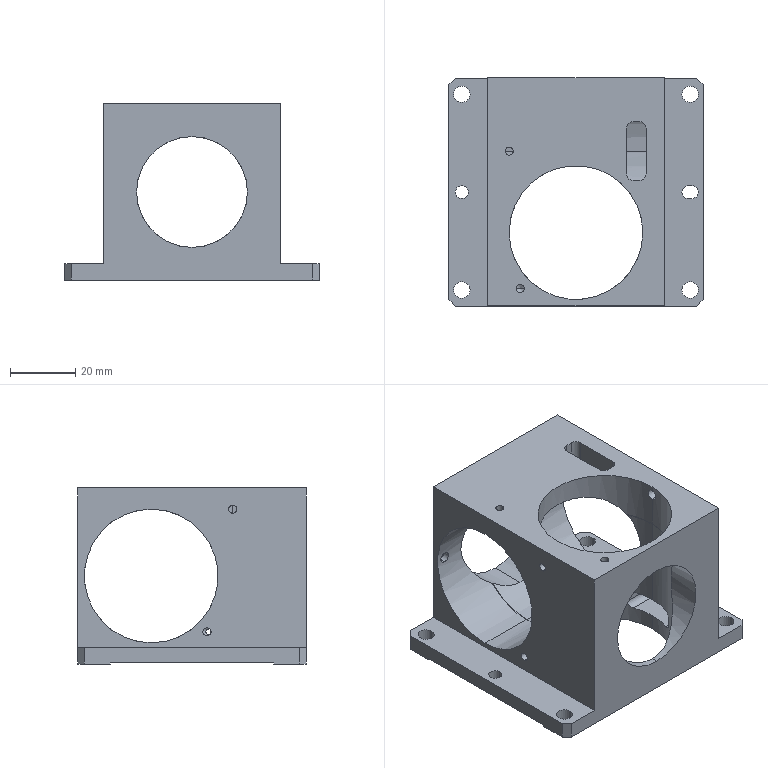NC program | NX | posted with a generic post | part box 78 x 70 x 54 mm
Whole program:
N10 G17 G21 G94 G90
(DRILLING_1_COPY_1_COPY_2 , TOOL : D6A45)
N12 T07 M6
N14 G54
N16 G17 G0 G90 X24. Y12.5 B0. C0. S5000 M3
N18 G43 Z30. H7
N20 G94 G81 G98 Z-13.75 F250. R-9.
N22 G80
N24 G0 X24. Y12.5 Z30.
N26 M5
(DRILLING_1_COPY_1_COPY_COPY , TOOL : 3.3ZT)
N28 T03 M6
N30 G54
N32 G17 G0 G90 X24. Y12.5 B0. C0. S2000 M3
N34 G43 Z30. H3
N36 G94 G83 G98 Z-21.058 F150. Q2. R-9.
N38 G80
N40 G0 X24. Y12.5 Z30.
N42 M5
(ZLEVEL_PROFILE_1_COPY , TOOL : D4)
N44 T04 M6
N46 G54
N48 G17 G0 G90 X-19.5 Y6.276 B0. C0. S9500 M3
N50 G43 Z30. H4
N52 Z-11.
N54 G94 G1 Y5.508 Z-11.04 F1250.
N56 X-19.49 Y5.5 Z-11.041
N58 X-17.529 Z-11.144
N60 X-17.5 Y5.507 Z-11.145
N62 Y19.453 Z-11.876
N64 X-17.509 Y19.5 Z-11.879
N66 X-19.491 Z-11.983
N68 X-19.5 Y19.453 Z-11.985
N70 Y12.504 Z-12.349
N72 Y5.508
N74 X-19.49 Y5.5
N76 X-17.529
N78 X-17.5 Y5.507
N80 Y19.453
N82 X-17.509 Y19.5
N84 X-19.491
N86 X-19.5 Y19.453
N88 Y12.504
N90 Y5.741 Z-12.467
N92 X-19.499 Y5.585 Z-12.47
N94 X-19.491 Y5.509 Z-12.471
N96 X-19.455 Y5.505 Z-12.472
N98 X-19.314 Y5.5 Z-12.475
N100 X-17.764 Z-12.502
N102 X-17.593 Z-12.505
N104 X-17.515 Y5.508 Z-12.506
N106 X-17.509 Y5.51
N108 X-17.507 Y5.524 Z-12.507
N110 X-17.5 Y5.665 Z-12.509
N112 Y16.513 Z-12.698
N114 Y19.453
N116 X-17.509 Y19.5
N118 X-19.491
N120 X-19.5 Y19.453
N122 Y12.504
N124 Y5.741 Z-12.816
N126 X-19.499 Y5.585 Z-12.819
N128 X-19.491 Y5.509 Z-12.821
N130 X-19.455 Y5.505
N132 X-19.314 Y5.5 Z-12.824
N134 X-17.764 Z-12.851
N136 X-17.593 Z-12.854
N138 X-17.515 Y5.508 Z-12.855
N140 X-17.509 Y5.51 Z-12.856
N142 X-17.507 Y5.524
N144 X-17.5 Y5.665 Z-12.858
N146 Y16.513 Z-13.048
N148 Y19.453
N150 X-17.509 Y19.5
N152 X-19.491
N154 X-19.5 Y19.453
N156 Y12.504
N158 Y5.741 Z-13.166
N160 X-19.499 Y5.585 Z-13.168
N162 X-19.491 Y5.509 Z-13.17
N164 X-19.455 Y5.505 Z-13.171
N166 X-19.314 Y5.5 Z-13.173
N168 X-17.764 Z-13.2
N170 X-17.593 Z-13.203
N172 X-17.515 Y5.508 Z-13.205
N174 X-17.509 Y5.51
N176 X-17.507 Y5.524
N178 X-17.5 Y5.665 Z-13.208
N180 Y16.513 Z-13.397
N182 Y19.453
N184 X-17.509 Y19.5
N186 X-19.491
N188 X-19.5 Y19.453
N190 Y12.504
N192 Y5.741 Z-13.515
N194 X-19.499 Y5.585 Z-13.518
N196 X-19.491 Y5.509 Z-13.519
N198 X-19.455 Y5.505 Z-13.52
N200 X-19.314 Y5.5 Z-13.522
N202 X-17.764 Z-13.549
N204 X-17.593 Z-13.552
N206 X-17.515 Y5.508 Z-13.554
N208 X-17.509 Y5.51
N210 X-17.507 Y5.524
N212 X-17.5 Y5.665 Z-13.557
N214 Y16.513 Z-13.746
N216 Y19.453
N218 X-17.51 Y19.5
N220 X-19.49
N222 X-19.5 Y19.453
N224 Y12.504
N226 Y5.741 Z-13.864
N228 X-19.499 Y5.585 Z-13.867
N230 X-19.491 Y5.509 Z-13.868
N232 X-19.455 Y5.505 Z-13.869
N234 X-19.314 Y5.5 Z-13.872
N236 X-17.764 Z-13.899
N238 X-17.593 Z-13.902
N240 X-17.515 Y5.508 Z-13.903
N242 X-17.509 Y5.51
N244 X-17.507 Y5.524
N246 X-17.5 Y5.665 Z-13.906
N248 Y16.513 Z-14.095
N250 Y19.453
N252 X-17.51 Y19.5
N254 X-19.49
N256 X-19.5 Y19.453
N258 Y12.504
N260 Y5.741 Z-14.213
N262 X-19.499 Y5.585 Z-14.216
N264 X-19.491 Y5.509 Z-14.218
N266 X-19.455 Y5.505
N268 X-19.314 Y5.5 Z-14.221
N270 X-17.764 Z-14.248
N272 X-17.593 Z-14.251
N274 X-17.515 Y5.508 Z-14.252
N276 X-17.509 Y5.51
N278 X-17.507 Y5.524 Z-14.253
N280 X-17.5 Y5.665 Z-14.255
N282 Y16.513 Z-14.445
N284 Y19.453
N286 X-17.51 Y19.5
N288 X-19.49
N290 X-19.5 Y19.453
N292 Y12.504
N294 Y5.741 Z-14.563
N296 X-19.499 Y5.585 Z-14.565
N298 X-19.491 Y5.509 Z-14.567
N300 X-19.455 Y5.505 Z-14.568
N302 X-19.314 Y5.5 Z-14.57
N304 X-17.764 Z-14.597
N306 X-17.593 Z-14.6
N308 X-17.515 Y5.508 Z-14.602
N310 X-17.509 Y5.509
N312 X-17.507 Y5.524
N314 X-17.5 Y5.665 Z-14.604
N316 Y16.514 Z-14.794
N318 Y19.453
N320 X-17.51 Y19.5
N322 X-19.49
N324 X-19.5 Y19.453
N326 Y12.504
N328 Y5.741 Z-14.912
N330 X-19.499 Y5.585 Z-14.915
N332 X-19.491 Y5.509 Z-14.916
N334 X-19.455 Y5.505 Z-14.917
N336 X-19.314 Y5.5 Z-14.919
N338 X-17.764 Z-14.946
N340 X-17.593 Z-14.949
N342 X-17.515 Y5.508 Z-14.951
N344 X-17.509 Y5.51
N346 X-17.507 Y5.524
N348 X-17.5 Y5.665 Z-14.954
N350 Y16.514 Z-15.143
N352 Y19.453
N354 X-17.51 Y19.5
N356 X-19.49
N358 X-19.5 Y19.453
N360 Y12.504
N362 Y5.741 Z-15.261
N364 X-19.499 Y5.585 Z-15.264
N366 X-19.491 Y5.509 Z-15.265
N368 X-19.455 Y5.505 Z-15.266
N370 X-19.314 Y5.5 Z-15.268
N372 X-17.764 Z-15.295
N374 X-17.593 Z-15.298
N376 X-17.515 Y5.508 Z-15.3
N378 X-17.509 Y5.51
N380 X-17.507 Y5.524
N382 X-17.5 Y5.665 Z-15.303
N384 Y16.514 Z-15.492
N386 Y19.453
N388 X-17.511 Y19.5
N390 X-19.489
N392 X-19.5 Y19.453
N394 Y12.504
N396 Y5.741 Z-15.61
N398 X-19.499 Y5.585 Z-15.613
N400 X-19.491 Y5.509 Z-15.614
N402 X-19.455 Y5.505 Z-15.615
N404 X-19.314 Y5.5 Z-15.618
N406 X-17.764 Z-15.645
N408 X-17.593 Z-15.648
N410 X-17.515 Y5.508 Z-15.649
N412 X-17.509 Y5.51
N414 X-17.507 Y5.524 Z-15.65
N416 X-17.5 Y5.665 Z-15.652
N418 Y16.514 Z-15.841
N420 Y19.453
N422 X-17.511 Y19.5
N424 X-19.489
N426 X-19.5 Y19.453
N428 Y12.504
N430 Y5.741 Z-15.959
N432 X-19.499 Y5.585 Z-15.962
N434 X-19.491 Y5.509 Z-15.964
N436 X-19.455 Y5.505
N438 X-19.314 Y5.5 Z-15.967
N440 X-17.764 Z-15.994
N442 X-17.593 Z-15.997
N444 X-17.515 Y5.508 Z-15.998
N446 X-17.509 Y5.51 Z-15.999
N448 X-17.507 Y5.524
N450 X-17.5 Y5.665 Z-16.001
N452 Y16.514 Z-16.191
N454 Y19.453
N456 X-17.511 Y19.5
N458 X-19.489
N460 X-19.5 Y19.453
N462 Y12.504
N464 Y5.741 Z-16.309
N466 X-19.499 Y5.585 Z-16.311
N468 X-19.491 Y5.509 Z-16.313
N470 X-19.455 Y5.505 Z-16.314
N472 X-19.314 Y5.5 Z-16.316
N474 X-17.764 Z-16.343
N476 X-17.593 Z-16.346
N478 X-17.515 Y5.508 Z-16.348
N480 X-17.509 Y5.51
N482 X-17.507 Y5.524
N484 X-17.5 Y5.665 Z-16.351
N486 Y16.514 Z-16.54
N488 Y19.453
N490 X-17.511 Y19.5
N492 X-19.489
N494 X-19.5 Y19.453
N496 Y12.504
N498 Y5.741 Z-16.658
N500 X-19.499 Y5.585 Z-16.661
N502 X-19.491 Y5.509 Z-16.662
N504 X-19.455 Y5.505 Z-16.663
N506 X-19.314 Y5.5 Z-16.665
N508 X-17.764 Z-16.692
N510 X-17.593 Z-16.695
N512 X-17.515 Y5.508 Z-16.697
N514 X-17.509 Y5.51
N516 X-17.507 Y5.524
N518 X-17.5 Y5.665 Z-16.7
N520 Y16.514 Z-16.889
N522 Y19.453
N524 X-17.512 Y19.5
N526 X-19.488
N528 X-19.5 Y19.453
N530 Y12.504
N532 Y5.741 Z-17.007
N534 X-19.499 Y5.585 Z-17.01
N536 X-19.491 Y5.509 Z-17.011
N538 X-19.455 Y5.505 Z-17.012
N540 X-19.314 Y5.5 Z-17.015
N542 X-17.764 Z-17.042
N544 X-17.593 Z-17.045
N546 X-17.515 Y5.508 Z-17.046
N548 X-17.509 Y5.51
N550 X-17.507 Y5.524
N552 X-17.5 Y5.665 Z-17.049
N554 Y16.514 Z-17.238
N556 Y19.453
N558 X-17.512 Y19.5
N560 X-19.488
N562 X-19.5 Y19.453
N564 Y12.504
N566 Y5.741 Z-17.356
N568 X-19.499 Y5.585 Z-17.359
N570 X-19.491 Y5.509 Z-17.361
N572 X-19.455 Y5.505
N574 X-19.314 Y5.5 Z-17.364
N576 X-17.764 Z-17.391
N578 X-17.593 Z-17.394
N580 X-17.515 Y5.508 Z-17.395
N582 X-17.509 Y5.51
N584 X-17.507 Y5.524 Z-17.396
N586 X-17.5 Y5.665 Z-17.398
N588 Y16.514 Z-17.588
N590 Y19.453
N592 X-17.512 Y19.5
N594 X-19.488
N596 X-19.5 Y19.453
N598 Y12.504
N600 Y5.741 Z-17.706
N602 X-19.499 Y5.585 Z-17.708
N604 X-19.491 Y5.509 Z-17.71
N606 X-19.455 Y5.505
N608 X-19.314 Y5.5 Z-17.713
N610 X-17.764 Z-17.74
N612 X-17.593 Z-17.743
N614 X-17.515 Y5.508 Z-17.745
N616 X-17.509 Y5.51
N618 X-17.507 Y5.524
N620 X-17.5 Y5.665 Z-17.747
N622 Y16.514 Z-17.937
N624 Y19.453
N626 X-17.512 Y19.5
N628 X-19.488
N630 X-19.5 Y19.453
N632 Y12.504
N634 Y5.741 Z-18.055
N636 X-19.499 Y5.585 Z-18.058
N638 X-19.491 Y5.509 Z-18.059
N640 X-19.455 Y5.505 Z-18.06
N642 X-19.314 Y5.5 Z-18.062
N644 X-17.764 Z-18.089
N646 X-17.593 Z-18.092
N648 X-17.515 Y5.508 Z-18.094
N650 X-17.509 Y5.51
N652 X-17.507 Y5.524
N654 X-17.5 Y5.665 Z-18.097
N656 Y16.514 Z-18.286
N658 Y19.453
N660 X-17.512 Y19.5
N662 X-19.488
N664 X-19.5 Y19.453
N666 Y12.504
N668 Y5.741 Z-18.404
N670 X-19.499 Y5.585 Z-18.407
N672 X-19.491 Y5.509 Z-18.408
N674 X-19.455 Y5.505 Z-18.409
N676 X-19.314 Y5.5 Z-18.411
N678 X-17.764 Z-18.438
N680 X-17.593 Z-18.441
N682 X-17.515 Y5.508 Z-18.443
N684 X-17.509 Y5.51
N686 X-17.507 Y5.524
N688 X-17.5 Y5.665 Z-18.446
N690 Y16.514 Z-18.635
N692 Y19.453
N694 X-17.512 Y19.5
N696 X-19.488
N698 X-19.5 Y19.453
N700 Y12.504
N702 Y5.741 Z-18.753
N704 X-19.499 Y5.585 Z-18.756
N706 X-19.491 Y5.509 Z-18.757
N708 X-19.455 Y5.505 Z-18.758
N710 X-19.314 Y5.5 Z-18.761
N712 X-17.764 Z-18.788
N714 X-17.593 Z-18.791
N716 X-17.515 Y5.508 Z-18.792
N718 X-17.509 Y5.51
N720 X-17.507 Y5.524 Z-18.793
N722 X-17.5 Y5.665 Z-18.795
N724 Y16.514 Z-18.984
N726 Y19.453
N728 X-17.512 Y19.5
N730 X-19.488
N732 X-19.5 Y19.453
N734 Y12.504
N736 Y5.741 Z-19.102
N738 X-19.499 Y5.585 Z-19.105
N740 X-19.491 Y5.509 Z-19.107
N742 X-19.455 Y5.505
N744 X-19.314 Y5.5 Z-19.11
N746 X-17.764 Z-19.137
N748 X-17.593 Z-19.14
N750 X-17.515 Y5.508 Z-19.141
N752 X-17.509 Y5.51 Z-19.142
N754 X-17.507 Y5.524
N756 X-17.5 Y5.665 Z-19.144
N758 Y16.514 Z-19.334
N760 Y19.453
N762 X-17.512 Y19.5
N764 X-19.488
N766 X-19.5 Y19.453
N768 Y12.504
N770 Y5.741 Z-19.452
N772 X-19.499 Y5.585 Z-19.454
N774 X-19.491 Y5.509 Z-19.456
N776 X-19.455 Y5.505 Z-19.457
N778 X-19.314 Y5.5 Z-19.459
N780 X-17.764 Z-19.486
N782 X-17.593 Z-19.489
N784 X-17.515 Y5.508 Z-19.491
N786 X-17.509 Y5.51
N788 X-17.507 Y5.524
N790 X-17.5 Y5.665 Z-19.493
N792 Y16.514 Z-19.683
N794 Y19.453
N796 X-17.512 Y19.5
N798 X-19.488
N800 X-19.5 Y19.453
N802 Y12.504
N804 Y5.741 Z-19.801
N806 X-19.499 Y5.585 Z-19.804
N808 X-19.491 Y5.509 Z-19.805
N810 X-19.455 Y5.505 Z-19.806
N812 X-19.314 Y5.5 Z-19.808
N814 X-17.764 Z-19.835
N816 X-17.593 Z-19.838
N818 X-17.515 Y5.508 Z-19.84
N820 X-17.509 Y5.51
N822 X-17.507 Y5.524
N824 X-17.5 Y5.665 Z-19.843
N826 Y16.514 Z-20.032
N828 Y19.453
N830 X-17.512 Y19.5
N832 X-19.488
N834 X-19.5 Y19.453
N836 Y12.504
N838 Y5.741 Z-20.15
N840 X-19.499 Y5.585 Z-20.153
N842 X-19.491 Y5.509 Z-20.154
N844 X-19.455 Y5.505 Z-20.155
N846 X-19.314 Y5.5 Z-20.157
N848 X-17.764 Z-20.185
N850 X-17.593 Z-20.188
N852 X-17.515 Y5.508 Z-20.189
N854 X-17.509 Y5.51
N856 X-17.507 Y5.524
N858 X-17.5 Y5.665 Z-20.192
N860 Y16.514 Z-20.381
N862 Y19.453
N864 X-17.512 Y19.5
N866 X-19.488
N868 X-19.5 Y19.453
N870 Y12.504
N872 Y5.741 Z-20.499
N874 X-19.499 Y5.585 Z-20.502
N876 X-19.491 Y5.509 Z-20.504
N878 X-19.455 Y5.505
N880 X-19.314 Y5.5 Z-20.507
N882 X-17.764 Z-20.534
N884 X-17.593 Z-20.537
N886 X-17.515 Y5.508 Z-20.538
N888 X-17.509 Y5.51
N890 X-17.507 Y5.524 Z-20.539
N892 X-17.5 Y5.665 Z-20.541
N894 Y16.514 Z-20.731
N896 Y19.453
N898 X-17.512 Y19.5
N900 X-19.488
N902 X-19.5 Y19.453
N904 Y12.504
N906 Y5.741 Z-20.849
N908 X-19.499 Y5.585 Z-20.851
N910 X-19.491 Y5.509 Z-20.853
N912 X-19.455 Y5.505
N914 X-19.314 Y5.5 Z-20.856
N916 X-17.764 Z-20.883
N918 X-17.593 Z-20.886
N920 X-17.515 Y5.508 Z-20.887
N922 X-17.509 Y5.51 Z-20.888
N924 X-17.507 Y5.524
N926 X-17.5 Y5.665 Z-20.89
N928 Y16.514 Z-21.08
N930 Y19.453
N932 X-17.512 Y19.5
N934 X-19.488
N936 X-19.5 Y19.453
N938 Y12.504
N940 Y5.741 Z-21.198
N942 X-19.499 Y5.585 Z-21.201
N944 X-19.491 Y5.509 Z-21.202
N946 X-19.455 Y5.505 Z-21.203
N948 X-19.314 Y5.5 Z-21.205
N950 X-17.764 Z-21.232
N952 X-17.593 Z-21.235
N954 X-17.515 Y5.508 Z-21.237
N956 X-17.509 Y5.51
N958 X-17.507 Y5.524
N960 X-17.5 Y5.665 Z-21.24
N962 Y16.514 Z-21.429
N964 Y19.453
N966 X-17.512 Y19.5
N968 X-19.488
N970 X-19.5 Y19.453
N972 Y5.508
N974 X-19.49 Y5.5
N976 X-17.547
N978 X-17.5 Y5.514
N980 Y16.514
N982 Z-20.429
N984 G0 Z30.
N986 M5
(TOOLCOMP_COPY_COPY , TOOL : D16JING)
N988 T13 M6
N990 G54
N992 G17 G0 G90 X0. Y-12.5 B0. C0. S9500 M3
N994 G43 Z30. H13
N996 Z-11.5
N998 G41 G94 G1 X-3.167 Y-21.403 F1000. D13
N1000 G3 X0. Y-25.15 R3.212
N1002 X0. Y-25.15 Z-16.5 I0. J12.65
N1004 X0. Y-25.15 Z-21.5 I0. J12.65
N1006 X0. Y-25.15 Z-26.5 I0. J12.65
N1008 X0. Y-25.15 Z-31.5 I0. J12.65
N1010 X0. Y-25.15 Z-36.5 I0. J12.65
N1012 X0. Y-25.15 Z-41.5 I0. J12.65
N1014 X0. Y-25.15 Z-46.5 I0. J12.65
N1016 X12.031 Y-8.591 Z-48. R12.65
N1018 X-3.909 Y-0.469 R12.65
N1020 X12.031 Y-8.591 R-12.65
N1022 X7.489 Y-6.737 R3.212
N1024 G40
N1026 G1 X0. Y-12.5
N1028 G0 Z30.
N1030 M5
N1032 M2